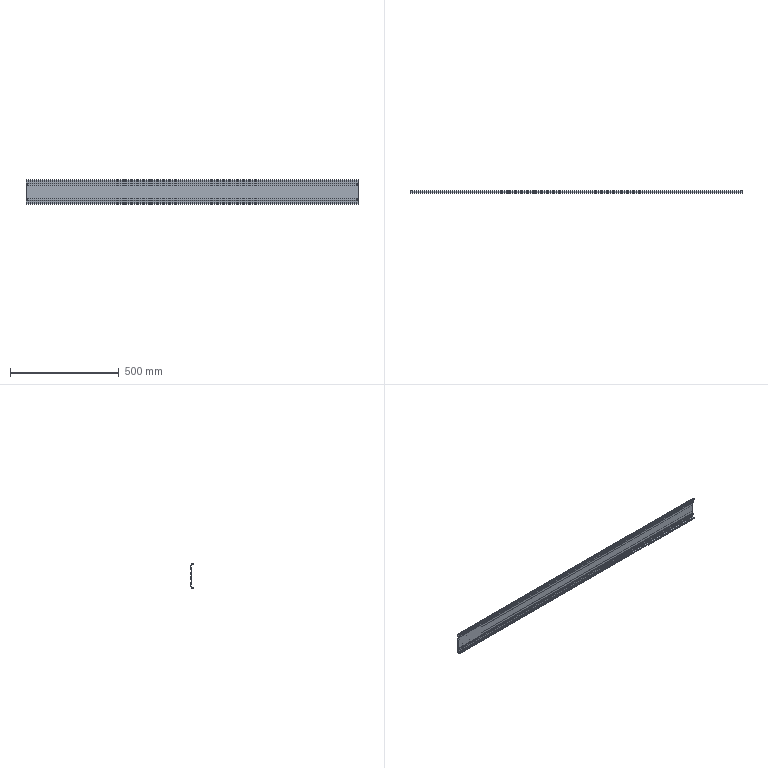Part | STEP file | SM140A-20-1140D-140A-600 Upper cover SF600 | 1 solid | 74 faces | box 1524 x 10 x 112 mm | volume 391118 mm3 | plane 38 | cylinder 36 | commonest cylinder face diameters 6 x12 2 x8 4 x8 0.98 x4 8 x4